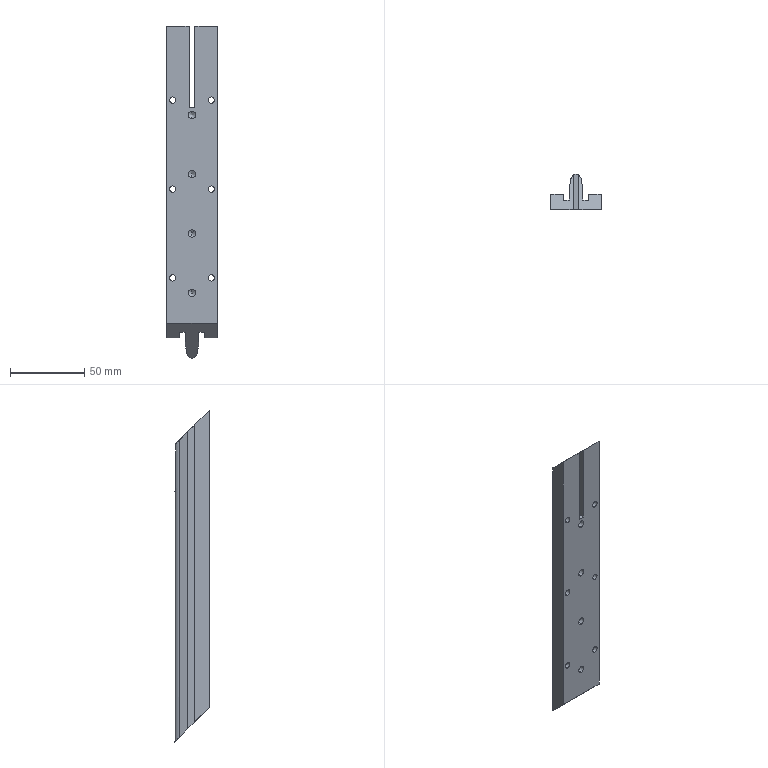Part | STEP file | slingshot track | 1 solid | 49 faces | box 34 x 23.53 x 224 mm | volume 76613 mm3 | cylinder 21 | plane 20 | cone 8 | commonest cylinder face diameters 4.2 x12 5 x8 6.8 x1